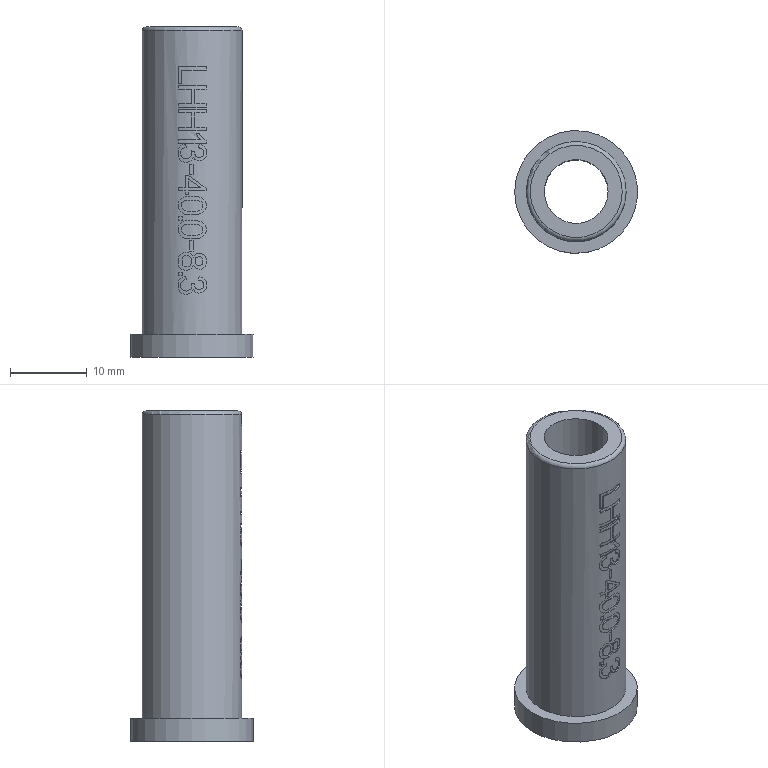Part | NX | features MI_LHH_0167 2 | 1 solid | 165 faces | box 16 x 16 x 43 mm | volume 3580 mm3 | plane 100 | cylinder 64 | torus 1 | commonest cylinder face diameters 12.8 x14 13 x6 2.135 x4 1.173 x2 1.254 x2 1.465 x2